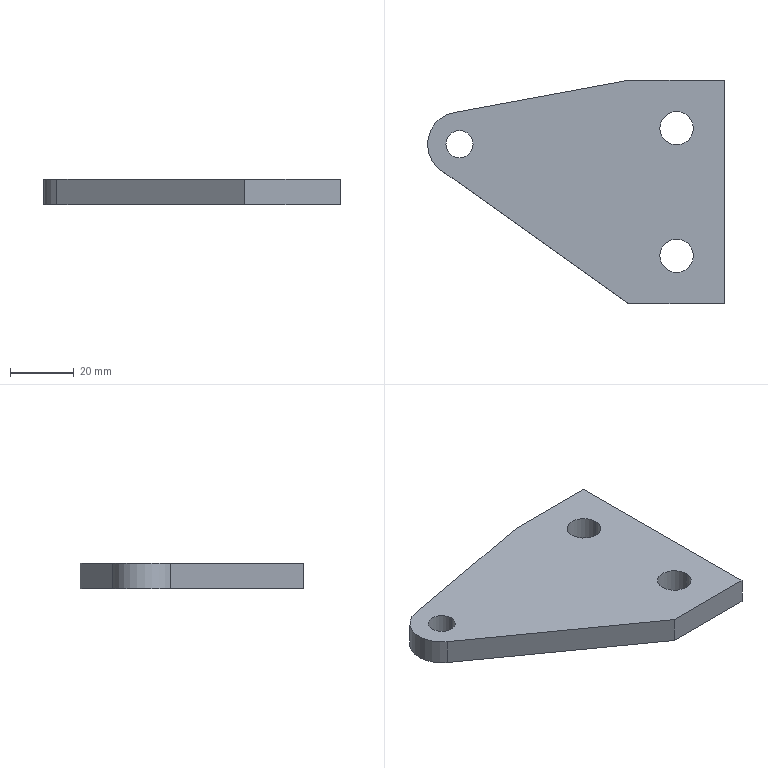Part | SolidWorks | features Extrusion 1, HoleWzd 1, ICE 1 | 1 solid | 14 faces | box 93 x 70 x 8 mm | volume 35854 mm3 | cylinder 7 | plane 7 | commonest cylinder face diameters 10.5 x4 8.5 x2 20 x1
STEP:
#1=CARTESIAN_POINT('',(-31.636,13.409,-4.));
#2=VERTEX_POINT('',#1);
#3=CARTESIAN_POINT('',(-23.136,13.409,-4.));
#4=VERTEX_POINT('',#3);
#5=CARTESIAN_POINT('',(-27.386,13.409,-4.));
#6=DIRECTION('',(0.,0.,1.));
#7=DIRECTION('',(1.,0.,0.));
#8=AXIS2_PLACEMENT_3D('',#5,#6,#7);
#9=CIRCLE('',#8,4.25);
#10=EDGE_CURVE('',#2,#4,#9,.T.);
#11=ORIENTED_EDGE('',*,*,#10,.F.);
#12=CARTESIAN_POINT('',(-31.636,13.409,4.));
#13=VERTEX_POINT('',#12);
#14=CARTESIAN_POINT('',(-31.636,13.409,4.));
#15=DIRECTION('',(0.,0.,1.));
#16=VECTOR('',#15,1000.);
#17=LINE('',#14,#16);
#18=EDGE_CURVE('',#2,#13,#17,.T.);
#19=ORIENTED_EDGE('',*,*,#18,.T.);
#20=CARTESIAN_POINT('',(-23.136,13.409,4.));
#21=VERTEX_POINT('',#20);
#22=CARTESIAN_POINT('',(-27.386,13.409,4.));
#23=DIRECTION('',(0.,0.,1.));
#24=DIRECTION('',(1.,0.,0.));
#25=AXIS2_PLACEMENT_3D('',#22,#23,#24);
#26=CIRCLE('',#25,4.25);
#27=EDGE_CURVE('',#13,#21,#26,.T.);
#28=ORIENTED_EDGE('',*,*,#27,.T.);
#29=CARTESIAN_POINT('',(-23.136,13.409,4.));
#30=DIRECTION('',(0.,0.,1.));
#31=VECTOR('',#30,1000.);
#32=LINE('',#29,#31);
#33=EDGE_CURVE('',#4,#21,#32,.T.);
#34=ORIENTED_EDGE('',*,*,#33,.F.);
#35=EDGE_LOOP('',(#11,#19,#28,#34));
#36=FACE_OUTER_BOUND('',#35,.T.);
#37=CARTESIAN_POINT('',(-27.386,13.409,4.));
#38=DIRECTION('',(0.,0.,1.));
#39=DIRECTION('',(1.,0.,0.));
#40=AXIS2_PLACEMENT_3D('',#37,#38,#39);
#41=CYLINDRICAL_SURFACE('',#40,4.25);
#42=ADVANCED_FACE('',(#36),#41,.F.);
#43=CARTESIAN_POINT('',(35.364,18.409,-4.));
#44=VERTEX_POINT('',#43);
#45=CARTESIAN_POINT('',(45.864,18.409,-4.));
#46=VERTEX_POINT('',#45);
#47=CARTESIAN_POINT('',(40.614,18.409,-4.));
#48=DIRECTION('',(0.,0.,1.));
#49=DIRECTION('',(-1.,0.,0.));
#50=AXIS2_PLACEMENT_3D('',#47,#48,#49);
#51=CIRCLE('',#50,5.25);
#52=EDGE_CURVE('',#44,#46,#51,.T.);
#53=ORIENTED_EDGE('',*,*,#52,.F.);
#54=CARTESIAN_POINT('',(35.364,18.409,4.));
#55=VERTEX_POINT('',#54);
#56=CARTESIAN_POINT('',(35.364,18.409,-4.));
#57=DIRECTION('',(0.,0.,1.));
#58=VECTOR('',#57,1000.);
#59=LINE('',#56,#58);
#60=EDGE_CURVE('',#44,#55,#59,.T.);
#61=ORIENTED_EDGE('',*,*,#60,.T.);
#62=CARTESIAN_POINT('',(45.864,18.409,4.));
#63=VERTEX_POINT('',#62);
#64=CARTESIAN_POINT('',(40.614,18.409,4.));
#65=DIRECTION('',(0.,0.,1.));
#66=DIRECTION('',(-1.,0.,0.));
#67=AXIS2_PLACEMENT_3D('',#64,#65,#66);
#68=CIRCLE('',#67,5.25);
#69=EDGE_CURVE('',#55,#63,#68,.T.);
#70=ORIENTED_EDGE('',*,*,#69,.T.);
#71=CARTESIAN_POINT('',(45.864,18.409,-4.));
#72=DIRECTION('',(0.,0.,1.));
#73=VECTOR('',#72,1000.);
#74=LINE('',#71,#73);
#75=EDGE_CURVE('',#46,#63,#74,.T.);
#76=ORIENTED_EDGE('',*,*,#75,.F.);
#77=EDGE_LOOP('',(#53,#61,#70,#76));
#78=FACE_OUTER_BOUND('',#77,.T.);
#79=CARTESIAN_POINT('',(40.614,18.409,-4.));
#80=DIRECTION('',(0.,0.,1.));
#81=DIRECTION('',(1.,0.,0.));
#82=AXIS2_PLACEMENT_3D('',#79,#80,#81);
#83=CYLINDRICAL_SURFACE('',#82,5.25);
#84=ADVANCED_FACE('',(#78),#83,.F.);
#85=CARTESIAN_POINT('',(35.364,-21.591,-4.));
#86=VERTEX_POINT('',#85);
#87=CARTESIAN_POINT('',(45.864,-21.591,-4.));
#88=VERTEX_POINT('',#87);
#89=CARTESIAN_POINT('',(40.614,-21.591,-4.));
#90=DIRECTION('',(0.,0.,1.));
#91=DIRECTION('',(-1.,0.,0.));
#92=AXIS2_PLACEMENT_3D('',#89,#90,#91);
#93=CIRCLE('',#92,5.25);
#94=EDGE_CURVE('',#86,#88,#93,.T.);
#95=ORIENTED_EDGE('',*,*,#94,.F.);
#96=CARTESIAN_POINT('',(35.364,-21.591,4.));
#97=VERTEX_POINT('',#96);
#98=CARTESIAN_POINT('',(35.364,-21.591,-4.));
#99=DIRECTION('',(0.,0.,1.));
#100=VECTOR('',#99,1000.);
#101=LINE('',#98,#100);
#102=EDGE_CURVE('',#86,#97,#101,.T.);
#103=ORIENTED_EDGE('',*,*,#102,.T.);
#104=CARTESIAN_POINT('',(45.864,-21.591,4.));
#105=VERTEX_POINT('',#104);
#106=CARTESIAN_POINT('',(40.614,-21.591,4.));
#107=DIRECTION('',(0.,0.,1.));
#108=DIRECTION('',(-1.,0.,0.));
#109=AXIS2_PLACEMENT_3D('',#106,#107,#108);
#110=CIRCLE('',#109,5.25);
#111=EDGE_CURVE('',#97,#105,#110,.T.);
#112=ORIENTED_EDGE('',*,*,#111,.T.);
#113=CARTESIAN_POINT('',(45.864,-21.591,-4.));
#114=DIRECTION('',(0.,0.,1.));
#115=VECTOR('',#114,1000.);
#116=LINE('',#113,#115);
#117=EDGE_CURVE('',#88,#105,#116,.T.);
#118=ORIENTED_EDGE('',*,*,#117,.F.);
#119=EDGE_LOOP('',(#95,#103,#112,#118));
#120=FACE_OUTER_BOUND('',#119,.T.);
#121=CARTESIAN_POINT('',(40.614,-21.591,-4.));
#122=DIRECTION('',(0.,0.,1.));
#123=DIRECTION('',(1.,0.,0.));
#124=AXIS2_PLACEMENT_3D('',#121,#122,#123);
#125=CYLINDRICAL_SURFACE('',#124,5.25);
#126=ADVANCED_FACE('',(#120),#125,.F.);
#127=CARTESIAN_POINT('',(25.614,-36.591,4.));
#128=VERTEX_POINT('',#127);
#129=CARTESIAN_POINT('',(55.614,-36.591,4.));
#130=VERTEX_POINT('',#129);
#131=CARTESIAN_POINT('',(-44.386,-36.591,4.));
#132=DIRECTION('',(1.,0.,0.));
#133=VECTOR('',#132,1000.);
#134=LINE('',#131,#133);
#135=EDGE_CURVE('',#128,#130,#134,.T.);
#136=ORIENTED_EDGE('',*,*,#135,.F.);
#137=CARTESIAN_POINT('',(25.614,-36.591,-4.));
#138=VERTEX_POINT('',#137);
#139=CARTESIAN_POINT('',(25.614,-36.591,-6.));
#140=DIRECTION('',(0.,0.,1.));
#141=VECTOR('',#140,1000.);
#142=LINE('',#139,#141);
#143=EDGE_CURVE('',#138,#128,#142,.T.);
#144=ORIENTED_EDGE('',*,*,#143,.F.);
#145=CARTESIAN_POINT('',(55.614,-36.591,-4.));
#146=VERTEX_POINT('',#145);
#147=CARTESIAN_POINT('',(-44.386,-36.591,-4.));
#148=DIRECTION('',(1.,0.,0.));
#149=VECTOR('',#148,1000.);
#150=LINE('',#147,#149);
#151=EDGE_CURVE('',#138,#146,#150,.T.);
#152=ORIENTED_EDGE('',*,*,#151,.T.);
#153=CARTESIAN_POINT('',(55.614,-36.591,-4.));
#154=DIRECTION('',(0.,0.,1.));
#155=VECTOR('',#154,1000.);
#156=LINE('',#153,#155);
#157=EDGE_CURVE('',#146,#130,#156,.T.);
#158=ORIENTED_EDGE('',*,*,#157,.T.);
#159=EDGE_LOOP('',(#136,#144,#152,#158));
#160=FACE_OUTER_BOUND('',#159,.T.);
#161=CARTESIAN_POINT('',(-44.386,-36.591,-4.));
#162=DIRECTION('',(0.,-1.,0.));
#163=DIRECTION('',(0.,0.,-1.));
#164=AXIS2_PLACEMENT_3D('',#161,#162,#163);
#165=PLANE('',#164);
#166=ADVANCED_FACE('',(#160),#165,.T.);
#167=CARTESIAN_POINT('',(55.614,33.409,-4.));
#168=VERTEX_POINT('',#167);
#169=CARTESIAN_POINT('',(25.614,33.409,-4.));
#170=VERTEX_POINT('',#169);
#171=CARTESIAN_POINT('',(55.614,33.409,-4.));
#172=DIRECTION('',(-1.,0.,0.));
#173=VECTOR('',#172,1000.);
#174=LINE('',#171,#173);
#175=EDGE_CURVE('',#168,#170,#174,.T.);
#176=ORIENTED_EDGE('',*,*,#175,.T.);
#177=CARTESIAN_POINT('',(25.614,33.409,4.));
#178=VERTEX_POINT('',#177);
#179=CARTESIAN_POINT('',(25.614,33.409,-6.));
#180=DIRECTION('',(0.,0.,1.));
#181=VECTOR('',#180,1000.);
#182=LINE('',#179,#181);
#183=EDGE_CURVE('',#170,#178,#182,.T.);
#184=ORIENTED_EDGE('',*,*,#183,.T.);
#185=CARTESIAN_POINT('',(55.614,33.409,4.));
#186=VERTEX_POINT('',#185);
#187=CARTESIAN_POINT('',(55.614,33.409,4.));
#188=DIRECTION('',(-1.,0.,0.));
#189=VECTOR('',#188,1000.);
#190=LINE('',#187,#189);
#191=EDGE_CURVE('',#186,#178,#190,.T.);
#192=ORIENTED_EDGE('',*,*,#191,.F.);
#193=CARTESIAN_POINT('',(55.614,33.409,-4.));
#194=DIRECTION('',(0.,0.,1.));
#195=VECTOR('',#194,1000.);
#196=LINE('',#193,#195);
#197=EDGE_CURVE('',#168,#186,#196,.T.);
#198=ORIENTED_EDGE('',*,*,#197,.F.);
#199=EDGE_LOOP('',(#176,#184,#192,#198));
#200=FACE_OUTER_BOUND('',#199,.T.);
#201=CARTESIAN_POINT('',(55.614,33.409,-4.));
#202=DIRECTION('',(0.,1.,0.));
#203=DIRECTION('',(-1.,0.,0.));
#204=AXIS2_PLACEMENT_3D('',#201,#202,#203);
#205=PLANE('',#204);
#206=ADVANCED_FACE('',(#200),#205,.T.);
#207=CARTESIAN_POINT('',(-27.386,13.409,-4.));
#208=DIRECTION('',(0.,0.,1.));
#209=DIRECTION('',(1.,0.,0.));
#210=AXIS2_PLACEMENT_3D('',#207,#208,#209);
#211=CIRCLE('',#210,4.25);
#212=EDGE_CURVE('',#4,#2,#211,.T.);
#213=ORIENTED_EDGE('',*,*,#212,.T.);
#214=ORIENTED_EDGE('',*,*,#10,.T.);
#215=EDGE_LOOP('',(#213,#214));
#216=FACE_BOUND('',#215,.T.);
#217=CARTESIAN_POINT('',(40.614,-21.591,-4.));
#218=DIRECTION('',(0.,0.,1.));
#219=DIRECTION('',(-1.,0.,0.));
#220=AXIS2_PLACEMENT_3D('',#217,#218,#219);
#221=CIRCLE('',#220,5.25);
#222=EDGE_CURVE('',#88,#86,#221,.T.);
#223=ORIENTED_EDGE('',*,*,#222,.T.);
#224=ORIENTED_EDGE('',*,*,#94,.T.);
#225=EDGE_LOOP('',(#223,#224));
#226=FACE_BOUND('',#225,.T.);
#227=CARTESIAN_POINT('',(40.614,18.409,-4.));
#228=DIRECTION('',(0.,0.,1.));
#229=DIRECTION('',(-1.,0.,0.));
#230=AXIS2_PLACEMENT_3D('',#227,#228,#229);
#231=CIRCLE('',#230,5.25);
#232=EDGE_CURVE('',#46,#44,#231,.T.);
#233=ORIENTED_EDGE('',*,*,#232,.T.);
#234=ORIENTED_EDGE('',*,*,#52,.T.);
#235=EDGE_LOOP('',(#233,#234));
#236=FACE_BOUND('',#235,.T.);
#237=CARTESIAN_POINT('',(-33.185,5.262,-4.));
#238=VERTEX_POINT('',#237);
#239=CARTESIAN_POINT('',(-8.674,-12.185,-4.));
#240=DIRECTION('',(0.8147,-0.5799,0.));
#241=VECTOR('',#240,1000.);
#242=LINE('',#239,#241);
#243=EDGE_CURVE('',#238,#138,#242,.T.);
#244=ORIENTED_EDGE('',*,*,#243,.F.);
#245=CARTESIAN_POINT('',(-29.21,23.241,-4.));
#246=VERTEX_POINT('',#245);
#247=CARTESIAN_POINT('',(-27.386,13.409,-4.));
#248=DIRECTION('',(0.,0.,1.));
#249=DIRECTION('',(1.,0.,0.));
#250=AXIS2_PLACEMENT_3D('',#247,#248,#249);
#251=CIRCLE('',#250,10.);
#252=EDGE_CURVE('',#246,#238,#251,.T.);
#253=ORIENTED_EDGE('',*,*,#252,.F.);
#254=CARTESIAN_POINT('',(-5.138,27.706,-4.));
#255=DIRECTION('',(-0.9832,-0.1824,0.));
#256=VECTOR('',#255,1000.);
#257=LINE('',#254,#256);
#258=EDGE_CURVE('',#170,#246,#257,.T.);
#259=ORIENTED_EDGE('',*,*,#258,.F.);
#260=ORIENTED_EDGE('',*,*,#175,.F.);
#261=CARTESIAN_POINT('',(55.614,-36.591,-4.));
#262=DIRECTION('',(0.,1.,0.));
#263=VECTOR('',#262,1000.);
#264=LINE('',#261,#263);
#265=EDGE_CURVE('',#146,#168,#264,.T.);
#266=ORIENTED_EDGE('',*,*,#265,.F.);
#267=ORIENTED_EDGE('',*,*,#151,.F.);
#268=EDGE_LOOP('',(#244,#253,#259,#260,#266,#267));
#269=FACE_OUTER_BOUND('',#268,.T.);
#270=CARTESIAN_POINT('',(0.,0.,-4.));
#271=DIRECTION('',(0.,0.,1.));
#272=DIRECTION('',(1.,0.,0.));
#273=AXIS2_PLACEMENT_3D('',#270,#271,#272);
#274=PLANE('',#273);
#275=ADVANCED_FACE('',(#216,#226,#236,#269),#274,.F.);
#276=CARTESIAN_POINT('',(-27.386,13.409,4.));
#277=DIRECTION('',(0.,0.,1.));
#278=DIRECTION('',(1.,0.,0.));
#279=AXIS2_PLACEMENT_3D('',#276,#277,#278);
#280=CIRCLE('',#279,4.25);
#281=EDGE_CURVE('',#21,#13,#280,.T.);
#282=ORIENTED_EDGE('',*,*,#281,.F.);
#283=ORIENTED_EDGE('',*,*,#27,.F.);
#284=EDGE_LOOP('',(#282,#283));
#285=FACE_BOUND('',#284,.T.);
#286=CARTESIAN_POINT('',(40.614,18.409,4.));
#287=DIRECTION('',(0.,0.,1.));
#288=DIRECTION('',(-1.,0.,0.));
#289=AXIS2_PLACEMENT_3D('',#286,#287,#288);
#290=CIRCLE('',#289,5.25);
#291=EDGE_CURVE('',#63,#55,#290,.T.);
#292=ORIENTED_EDGE('',*,*,#291,.F.);
#293=ORIENTED_EDGE('',*,*,#69,.F.);
#294=EDGE_LOOP('',(#292,#293));
#295=FACE_BOUND('',#294,.T.);
#296=CARTESIAN_POINT('',(40.614,-21.591,4.));
#297=DIRECTION('',(0.,0.,1.));
#298=DIRECTION('',(-1.,0.,0.));
#299=AXIS2_PLACEMENT_3D('',#296,#297,#298);
#300=CIRCLE('',#299,5.25);
#301=EDGE_CURVE('',#105,#97,#300,.T.);
#302=ORIENTED_EDGE('',*,*,#301,.F.);
#303=ORIENTED_EDGE('',*,*,#111,.F.);
#304=EDGE_LOOP('',(#302,#303));
#305=FACE_BOUND('',#304,.T.);
#306=CARTESIAN_POINT('',(-29.21,23.241,4.));
#307=VERTEX_POINT('',#306);
#308=CARTESIAN_POINT('',(-33.185,5.262,4.));
#309=VERTEX_POINT('',#308);
#310=CARTESIAN_POINT('',(-27.386,13.409,4.));
#311=DIRECTION('',(0.,0.,1.));
#312=DIRECTION('',(1.,0.,0.));
#313=AXIS2_PLACEMENT_3D('',#310,#311,#312);
#314=CIRCLE('',#313,10.);
#315=EDGE_CURVE('',#307,#309,#314,.T.);
#316=ORIENTED_EDGE('',*,*,#315,.T.);
#317=CARTESIAN_POINT('',(-33.185,5.262,4.));
#318=DIRECTION('',(0.8147,-0.5799,0.));
#319=VECTOR('',#318,1000.);
#320=LINE('',#317,#319);
#321=EDGE_CURVE('',#309,#128,#320,.T.);
#322=ORIENTED_EDGE('',*,*,#321,.T.);
#323=ORIENTED_EDGE('',*,*,#135,.T.);
#324=CARTESIAN_POINT('',(55.614,-36.591,4.));
#325=DIRECTION('',(0.,1.,0.));
#326=VECTOR('',#325,1000.);
#327=LINE('',#324,#326);
#328=EDGE_CURVE('',#130,#186,#327,.T.);
#329=ORIENTED_EDGE('',*,*,#328,.T.);
#330=ORIENTED_EDGE('',*,*,#191,.T.);
#331=CARTESIAN_POINT('',(25.614,33.409,4.));
#332=DIRECTION('',(-0.9832,-0.1824,0.));
#333=VECTOR('',#332,1000.);
#334=LINE('',#331,#333);
#335=EDGE_CURVE('',#178,#307,#334,.T.);
#336=ORIENTED_EDGE('',*,*,#335,.T.);
#337=EDGE_LOOP('',(#316,#322,#323,#329,#330,#336));
#338=FACE_OUTER_BOUND('',#337,.T.);
#339=CARTESIAN_POINT('',(0.,0.,4.));
#340=DIRECTION('',(0.,0.,1.));
#341=DIRECTION('',(1.,0.,0.));
#342=AXIS2_PLACEMENT_3D('',#339,#340,#341);
#343=PLANE('',#342);
#344=ADVANCED_FACE('',(#285,#295,#305,#338),#343,.T.);
#345=ORIENTED_EDGE('',*,*,#328,.F.);
#346=ORIENTED_EDGE('',*,*,#157,.F.);
#347=ORIENTED_EDGE('',*,*,#265,.T.);
#348=ORIENTED_EDGE('',*,*,#197,.T.);
#349=EDGE_LOOP('',(#345,#346,#347,#348));
#350=FACE_OUTER_BOUND('',#349,.T.);
#351=CARTESIAN_POINT('',(55.614,-36.591,-4.));
#352=DIRECTION('',(1.,0.,0.));
#353=DIRECTION('',(0.,0.,-1.));
#354=AXIS2_PLACEMENT_3D('',#351,#352,#353);
#355=PLANE('',#354);
#356=ADVANCED_FACE('',(#350),#355,.T.);
#357=ORIENTED_EDGE('',*,*,#102,.F.);
#358=ORIENTED_EDGE('',*,*,#222,.F.);
#359=ORIENTED_EDGE('',*,*,#117,.T.);
#360=ORIENTED_EDGE('',*,*,#301,.T.);
#361=EDGE_LOOP('',(#357,#358,#359,#360));
#362=FACE_OUTER_BOUND('',#361,.T.);
#363=CARTESIAN_POINT('',(40.614,-21.591,-4.));
#364=DIRECTION('',(0.,0.,1.));
#365=DIRECTION('',(1.,0.,0.));
#366=AXIS2_PLACEMENT_3D('',#363,#364,#365);
#367=CYLINDRICAL_SURFACE('',#366,5.25);
#368=ADVANCED_FACE('',(#362),#367,.F.);
#369=ORIENTED_EDGE('',*,*,#60,.F.);
#370=ORIENTED_EDGE('',*,*,#232,.F.);
#371=ORIENTED_EDGE('',*,*,#75,.T.);
#372=ORIENTED_EDGE('',*,*,#291,.T.);
#373=EDGE_LOOP('',(#369,#370,#371,#372));
#374=FACE_OUTER_BOUND('',#373,.T.);
#375=CARTESIAN_POINT('',(40.614,18.409,-4.));
#376=DIRECTION('',(0.,0.,1.));
#377=DIRECTION('',(1.,0.,0.));
#378=AXIS2_PLACEMENT_3D('',#375,#376,#377);
#379=CYLINDRICAL_SURFACE('',#378,5.25);
#380=ADVANCED_FACE('',(#374),#379,.F.);
#381=ORIENTED_EDGE('',*,*,#243,.T.);
#382=ORIENTED_EDGE('',*,*,#143,.T.);
#383=ORIENTED_EDGE('',*,*,#321,.F.);
#384=CARTESIAN_POINT('',(-33.185,5.262,-6.));
#385=DIRECTION('',(0.,0.,1.));
#386=VECTOR('',#385,1000.);
#387=LINE('',#384,#386);
#388=EDGE_CURVE('',#238,#309,#387,.T.);
#389=ORIENTED_EDGE('',*,*,#388,.F.);
#390=EDGE_LOOP('',(#381,#382,#383,#389));
#391=FACE_OUTER_BOUND('',#390,.T.);
#392=CARTESIAN_POINT('',(-33.185,5.262,-6.));
#393=DIRECTION('',(-0.5799,-0.8147,0.));
#394=DIRECTION('',(0.8147,-0.5799,0.));
#395=AXIS2_PLACEMENT_3D('',#392,#393,#394);
#396=PLANE('',#395);
#397=ADVANCED_FACE('',(#391),#396,.T.);
#398=ORIENTED_EDGE('',*,*,#252,.T.);
#399=ORIENTED_EDGE('',*,*,#388,.T.);
#400=ORIENTED_EDGE('',*,*,#315,.F.);
#401=CARTESIAN_POINT('',(-29.21,23.241,-6.));
#402=DIRECTION('',(0.,0.,1.));
#403=VECTOR('',#402,1000.);
#404=LINE('',#401,#403);
#405=EDGE_CURVE('',#246,#307,#404,.T.);
#406=ORIENTED_EDGE('',*,*,#405,.F.);
#407=EDGE_LOOP('',(#398,#399,#400,#406));
#408=FACE_OUTER_BOUND('',#407,.T.);
#409=CARTESIAN_POINT('',(-27.386,13.409,-6.));
#410=DIRECTION('',(0.,0.,1.));
#411=DIRECTION('',(1.,0.,0.));
#412=AXIS2_PLACEMENT_3D('',#409,#410,#411);
#413=CYLINDRICAL_SURFACE('',#412,10.);
#414=ADVANCED_FACE('',(#408),#413,.T.);
#415=ORIENTED_EDGE('',*,*,#258,.T.);
#416=ORIENTED_EDGE('',*,*,#405,.T.);
#417=ORIENTED_EDGE('',*,*,#335,.F.);
#418=ORIENTED_EDGE('',*,*,#183,.F.);
#419=EDGE_LOOP('',(#415,#416,#417,#418));
#420=FACE_OUTER_BOUND('',#419,.T.);
#421=CARTESIAN_POINT('',(25.614,33.409,-6.));
#422=DIRECTION('',(-0.1824,0.9832,0.));
#423=DIRECTION('',(-0.9832,-0.1824,0.));
#424=AXIS2_PLACEMENT_3D('',#421,#422,#423);
#425=PLANE('',#424);
#426=ADVANCED_FACE('',(#420),#425,.T.);
#427=ORIENTED_EDGE('',*,*,#18,.F.);
#428=ORIENTED_EDGE('',*,*,#212,.F.);
#429=ORIENTED_EDGE('',*,*,#33,.T.);
#430=ORIENTED_EDGE('',*,*,#281,.T.);
#431=EDGE_LOOP('',(#427,#428,#429,#430));
#432=FACE_OUTER_BOUND('',#431,.T.);
#433=CARTESIAN_POINT('',(-27.386,13.409,4.));
#434=DIRECTION('',(0.,0.,1.));
#435=DIRECTION('',(1.,0.,0.));
#436=AXIS2_PLACEMENT_3D('',#433,#434,#435);
#437=CYLINDRICAL_SURFACE('',#436,4.25);
#438=ADVANCED_FACE('',(#432),#437,.F.);
#439=CLOSED_SHELL('',(#42,#84,#126,#166,#206,#275,#344,#356,#368,#380,#397,#414,#426,#438));
#440=MANIFOLD_SOLID_BREP('',#439);
#441=CARTESIAN_POINT('',(0.,0.,0.));
#442=DIRECTION('',(0.,0.,1.));
#443=DIRECTION('',(1.,0.,0.));
#444=AXIS2_PLACEMENT_3D('',#441,#442,#443);
#445=(LENGTH_UNIT()NAMED_UNIT(*)SI_UNIT(.MILLI.,.METRE.));
#446=UNCERTAINTY_MEASURE_WITH_UNIT(LENGTH_MEASURE(0.00001),#445,'','');
#447=(NAMED_UNIT(*)PLANE_ANGLE_UNIT()SI_UNIT($,.RADIAN.));
#448=(NAMED_UNIT(*)SI_UNIT($,.STERADIAN.)SOLID_ANGLE_UNIT());
#449=(GEOMETRIC_REPRESENTATION_CONTEXT(3)GLOBAL_UNCERTAINTY_ASSIGNED_CONTEXT((#446))GLOBAL_UNIT_ASSIGNED_CONTEXT((#445,#447,#448))REPRESENTATION_CONTEXT('',''));
#450=ADVANCED_BREP_SHAPE_REPRESENTATION('',(#440,#444),#449);